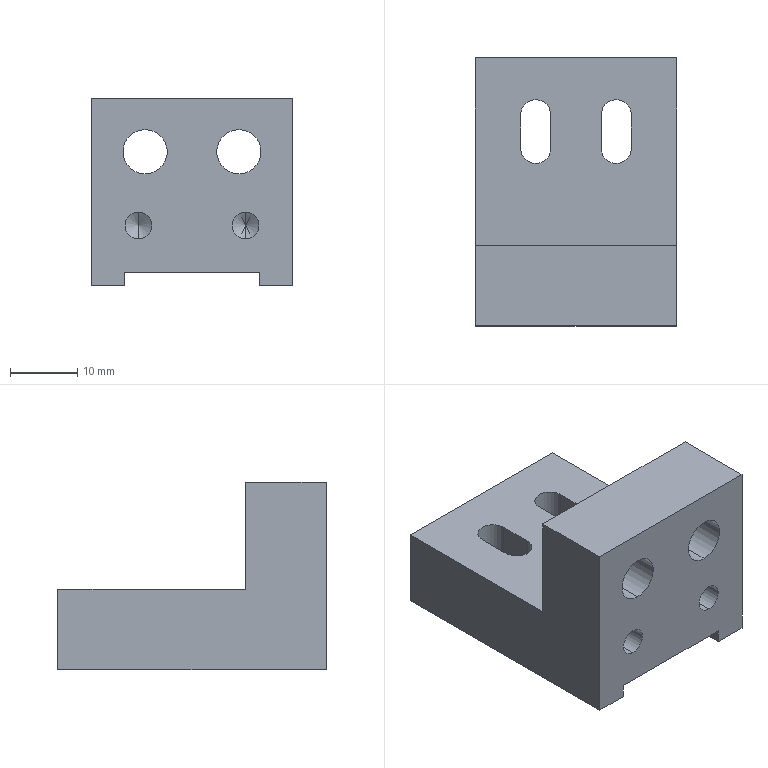Part | SolidWorks | features HoleWzd 4, ICE 3, Extrusion 1 | 1 solid | 38 faces | box 30 x 40 x 28 mm | volume 15981 mm3 | plane 18 | cylinder 16 | cone 4 | commonest cylinder face diameters 4 x4 4.5 x4 6.6 x4 11 x4
STEP:
#1=CARTESIAN_POINT('',(-7.,-14.4,14.5));
#2=VERTEX_POINT('',#1);
#3=CARTESIAN_POINT('',(-7.,-14.4,25.5));
#4=VERTEX_POINT('',#3);
#5=CARTESIAN_POINT('',(-7.,-14.4,20.));
#6=DIRECTION('',(0.,1.,0.));
#7=DIRECTION('',(0.,0.,1.));
#8=AXIS2_PLACEMENT_3D('',#5,#6,#7);
#9=CIRCLE('',#8,5.5);
#10=EDGE_CURVE('',#2,#4,#9,.T.);
#11=ORIENTED_EDGE('',*,*,#10,.F.);
#12=CARTESIAN_POINT('',(-7.,-8.,14.5));
#13=VERTEX_POINT('',#12);
#14=CARTESIAN_POINT('',(-7.,-8.,14.5));
#15=DIRECTION('',(0.,1.,0.));
#16=VECTOR('',#15,1000.);
#17=LINE('',#14,#16);
#18=EDGE_CURVE('',#2,#13,#17,.T.);
#19=ORIENTED_EDGE('',*,*,#18,.T.);
#20=CARTESIAN_POINT('',(-7.,-8.,25.5));
#21=VERTEX_POINT('',#20);
#22=CARTESIAN_POINT('',(-7.,-8.,20.));
#23=DIRECTION('',(0.,1.,0.));
#24=DIRECTION('',(0.,0.,1.));
#25=AXIS2_PLACEMENT_3D('',#22,#23,#24);
#26=CIRCLE('',#25,5.5);
#27=EDGE_CURVE('',#13,#21,#26,.T.);
#28=ORIENTED_EDGE('',*,*,#27,.T.);
#29=CARTESIAN_POINT('',(-7.,-8.,25.5));
#30=DIRECTION('',(0.,1.,0.));
#31=VECTOR('',#30,1000.);
#32=LINE('',#29,#31);
#33=EDGE_CURVE('',#4,#21,#32,.T.);
#34=ORIENTED_EDGE('',*,*,#33,.F.);
#35=EDGE_LOOP('',(#11,#19,#28,#34));
#36=FACE_OUTER_BOUND('',#35,.T.);
#37=CARTESIAN_POINT('',(-7.,-8.,20.));
#38=DIRECTION('',(0.,1.,0.));
#39=DIRECTION('',(0.,0.,1.));
#40=AXIS2_PLACEMENT_3D('',#37,#38,#39);
#41=CYLINDRICAL_SURFACE('',#40,5.5);
#42=ADVANCED_FACE('',(#36),#41,.F.);
#43=CARTESIAN_POINT('',(-7.,-20.,16.7));
#44=VERTEX_POINT('',#43);
#45=CARTESIAN_POINT('',(-7.,-20.,23.3));
#46=VERTEX_POINT('',#45);
#47=CARTESIAN_POINT('',(-7.,-20.,20.));
#48=DIRECTION('',(0.,1.,0.));
#49=DIRECTION('',(0.,0.,1.));
#50=AXIS2_PLACEMENT_3D('',#47,#48,#49);
#51=CIRCLE('',#50,3.3);
#52=EDGE_CURVE('',#44,#46,#51,.T.);
#53=ORIENTED_EDGE('',*,*,#52,.F.);
#54=CARTESIAN_POINT('',(-7.,-14.4,16.7));
#55=VERTEX_POINT('',#54);
#56=CARTESIAN_POINT('',(-7.,-8.,16.7));
#57=DIRECTION('',(0.,1.,0.));
#58=VECTOR('',#57,1000.);
#59=LINE('',#56,#58);
#60=EDGE_CURVE('',#44,#55,#59,.T.);
#61=ORIENTED_EDGE('',*,*,#60,.T.);
#62=CARTESIAN_POINT('',(-7.,-14.4,23.3));
#63=VERTEX_POINT('',#62);
#64=CARTESIAN_POINT('',(-7.,-14.4,20.));
#65=DIRECTION('',(0.,1.,0.));
#66=DIRECTION('',(0.,0.,1.));
#67=AXIS2_PLACEMENT_3D('',#64,#65,#66);
#68=CIRCLE('',#67,3.3);
#69=EDGE_CURVE('',#55,#63,#68,.T.);
#70=ORIENTED_EDGE('',*,*,#69,.T.);
#71=CARTESIAN_POINT('',(-7.,-8.,23.3));
#72=DIRECTION('',(0.,1.,0.));
#73=VECTOR('',#72,1000.);
#74=LINE('',#71,#73);
#75=EDGE_CURVE('',#46,#63,#74,.T.);
#76=ORIENTED_EDGE('',*,*,#75,.F.);
#77=EDGE_LOOP('',(#53,#61,#70,#76));
#78=FACE_OUTER_BOUND('',#77,.T.);
#79=CARTESIAN_POINT('',(-7.,-8.,20.));
#80=DIRECTION('',(0.,1.,0.));
#81=DIRECTION('',(0.,0.,1.));
#82=AXIS2_PLACEMENT_3D('',#79,#80,#81);
#83=CYLINDRICAL_SURFACE('',#82,3.3);
#84=ADVANCED_FACE('',(#78),#83,.F.);
#85=CARTESIAN_POINT('',(7.,-14.4,14.5));
#86=VERTEX_POINT('',#85);
#87=CARTESIAN_POINT('',(7.,-14.4,25.5));
#88=VERTEX_POINT('',#87);
#89=CARTESIAN_POINT('',(7.,-14.4,20.));
#90=DIRECTION('',(0.,1.,0.));
#91=DIRECTION('',(0.,0.,1.));
#92=AXIS2_PLACEMENT_3D('',#89,#90,#91);
#93=CIRCLE('',#92,5.5);
#94=EDGE_CURVE('',#86,#88,#93,.T.);
#95=ORIENTED_EDGE('',*,*,#94,.F.);
#96=CARTESIAN_POINT('',(7.,-8.,14.5));
#97=VERTEX_POINT('',#96);
#98=CARTESIAN_POINT('',(7.,-8.,14.5));
#99=DIRECTION('',(0.,1.,0.));
#100=VECTOR('',#99,1000.);
#101=LINE('',#98,#100);
#102=EDGE_CURVE('',#86,#97,#101,.T.);
#103=ORIENTED_EDGE('',*,*,#102,.T.);
#104=CARTESIAN_POINT('',(7.,-8.,25.5));
#105=VERTEX_POINT('',#104);
#106=CARTESIAN_POINT('',(7.,-8.,20.));
#107=DIRECTION('',(0.,1.,0.));
#108=DIRECTION('',(0.,0.,1.));
#109=AXIS2_PLACEMENT_3D('',#106,#107,#108);
#110=CIRCLE('',#109,5.5);
#111=EDGE_CURVE('',#97,#105,#110,.T.);
#112=ORIENTED_EDGE('',*,*,#111,.T.);
#113=CARTESIAN_POINT('',(7.,-8.,25.5));
#114=DIRECTION('',(0.,1.,0.));
#115=VECTOR('',#114,1000.);
#116=LINE('',#113,#115);
#117=EDGE_CURVE('',#88,#105,#116,.T.);
#118=ORIENTED_EDGE('',*,*,#117,.F.);
#119=EDGE_LOOP('',(#95,#103,#112,#118));
#120=FACE_OUTER_BOUND('',#119,.T.);
#121=CARTESIAN_POINT('',(7.,-8.,20.));
#122=DIRECTION('',(0.,1.,0.));
#123=DIRECTION('',(0.,0.,1.));
#124=AXIS2_PLACEMENT_3D('',#121,#122,#123);
#125=CYLINDRICAL_SURFACE('',#124,5.5);
#126=ADVANCED_FACE('',(#120),#125,.F.);
#127=CARTESIAN_POINT('',(7.,-20.,16.7));
#128=VERTEX_POINT('',#127);
#129=CARTESIAN_POINT('',(7.,-20.,23.3));
#130=VERTEX_POINT('',#129);
#131=CARTESIAN_POINT('',(7.,-20.,20.));
#132=DIRECTION('',(0.,1.,0.));
#133=DIRECTION('',(0.,0.,1.));
#134=AXIS2_PLACEMENT_3D('',#131,#132,#133);
#135=CIRCLE('',#134,3.3);
#136=EDGE_CURVE('',#128,#130,#135,.T.);
#137=ORIENTED_EDGE('',*,*,#136,.F.);
#138=CARTESIAN_POINT('',(7.,-14.4,16.7));
#139=VERTEX_POINT('',#138);
#140=CARTESIAN_POINT('',(7.,-8.,16.7));
#141=DIRECTION('',(0.,1.,0.));
#142=VECTOR('',#141,1000.);
#143=LINE('',#140,#142);
#144=EDGE_CURVE('',#128,#139,#143,.T.);
#145=ORIENTED_EDGE('',*,*,#144,.T.);
#146=CARTESIAN_POINT('',(7.,-14.4,23.3));
#147=VERTEX_POINT('',#146);
#148=CARTESIAN_POINT('',(7.,-14.4,20.));
#149=DIRECTION('',(0.,1.,0.));
#150=DIRECTION('',(0.,0.,1.));
#151=AXIS2_PLACEMENT_3D('',#148,#149,#150);
#152=CIRCLE('',#151,3.3);
#153=EDGE_CURVE('',#139,#147,#152,.T.);
#154=ORIENTED_EDGE('',*,*,#153,.T.);
#155=CARTESIAN_POINT('',(7.,-8.,23.3));
#156=DIRECTION('',(0.,1.,0.));
#157=VECTOR('',#156,1000.);
#158=LINE('',#155,#157);
#159=EDGE_CURVE('',#130,#147,#158,.T.);
#160=ORIENTED_EDGE('',*,*,#159,.F.);
#161=EDGE_LOOP('',(#137,#145,#154,#160));
#162=FACE_OUTER_BOUND('',#161,.T.);
#163=CARTESIAN_POINT('',(7.,-8.,20.));
#164=DIRECTION('',(0.,1.,0.));
#165=DIRECTION('',(0.,0.,1.));
#166=AXIS2_PLACEMENT_3D('',#163,#164,#165);
#167=CYLINDRICAL_SURFACE('',#166,3.3);
#168=ADVANCED_FACE('',(#162),#167,.F.);
#169=CARTESIAN_POINT('',(8.,-12.,11.));
#170=VERTEX_POINT('',#169);
#171=CARTESIAN_POINT('',(8.,-12.,7.));
#172=VERTEX_POINT('',#171);
#173=CARTESIAN_POINT('',(8.,-12.,9.));
#174=DIRECTION('',(0.,-1.,0.));
#175=DIRECTION('',(0.,0.,-1.));
#176=AXIS2_PLACEMENT_3D('',#173,#174,#175);
#177=CIRCLE('',#176,2.);
#178=EDGE_CURVE('',#170,#172,#177,.T.);
#179=ORIENTED_EDGE('',*,*,#178,.F.);
#180=CARTESIAN_POINT('',(8.,-20.,11.));
#181=VERTEX_POINT('',#180);
#182=CARTESIAN_POINT('',(8.,-20.,11.));
#183=DIRECTION('',(0.,-1.,0.));
#184=VECTOR('',#183,1000.);
#185=LINE('',#182,#184);
#186=EDGE_CURVE('',#170,#181,#185,.T.);
#187=ORIENTED_EDGE('',*,*,#186,.T.);
#188=CARTESIAN_POINT('',(8.,-20.,7.));
#189=VERTEX_POINT('',#188);
#190=CARTESIAN_POINT('',(8.,-20.,9.));
#191=DIRECTION('',(0.,-1.,0.));
#192=DIRECTION('',(0.,0.,-1.));
#193=AXIS2_PLACEMENT_3D('',#190,#191,#192);
#194=CIRCLE('',#193,2.);
#195=EDGE_CURVE('',#181,#189,#194,.T.);
#196=ORIENTED_EDGE('',*,*,#195,.T.);
#197=CARTESIAN_POINT('',(8.,-20.,7.));
#198=DIRECTION('',(0.,-1.,0.));
#199=VECTOR('',#198,1000.);
#200=LINE('',#197,#199);
#201=EDGE_CURVE('',#172,#189,#200,.T.);
#202=ORIENTED_EDGE('',*,*,#201,.F.);
#203=EDGE_LOOP('',(#179,#187,#196,#202));
#204=FACE_OUTER_BOUND('',#203,.T.);
#205=CARTESIAN_POINT('',(8.,-20.,9.));
#206=DIRECTION('',(0.,-1.,0.));
#207=DIRECTION('',(0.,0.,-1.));
#208=AXIS2_PLACEMENT_3D('',#205,#206,#207);
#209=CYLINDRICAL_SURFACE('',#208,2.);
#210=ADVANCED_FACE('',(#204),#209,.F.);
#211=CARTESIAN_POINT('',(8.,-10.798,9.));
#212=VERTEX_POINT('',#211);
#213=CARTESIAN_POINT('',(8.,-12.,7.));
#214=DIRECTION('',(0.,-0.515,-0.8572));
#215=VECTOR('',#214,1000.);
#216=LINE('',#213,#215);
#217=EDGE_CURVE('',#212,#172,#216,.T.);
#218=ORIENTED_EDGE('',*,*,#217,.F.);
#219=CARTESIAN_POINT('',(8.,-12.,11.));
#220=DIRECTION('',(0.,-0.515,0.8572));
#221=VECTOR('',#220,1000.);
#222=LINE('',#219,#221);
#223=EDGE_CURVE('',#212,#170,#222,.T.);
#224=ORIENTED_EDGE('',*,*,#223,.T.);
#225=ORIENTED_EDGE('',*,*,#178,.T.);
#226=EDGE_LOOP('',(#218,#224,#225));
#227=FACE_OUTER_BOUND('',#226,.T.);
#228=CARTESIAN_POINT('',(8.,-12.,9.));
#229=DIRECTION('',(0.,-1.,0.));
#230=DIRECTION('',(0.,0.,-1.));
#231=AXIS2_PLACEMENT_3D('',#228,#229,#230);
#232=CONICAL_SURFACE('',#231,2.,1.03);
#233=ADVANCED_FACE('',(#227),#232,.F.);
#234=CARTESIAN_POINT('',(-8.,-12.,11.));
#235=VERTEX_POINT('',#234);
#236=CARTESIAN_POINT('',(-8.,-12.,7.));
#237=VERTEX_POINT('',#236);
#238=CARTESIAN_POINT('',(-8.,-12.,9.));
#239=DIRECTION('',(0.,-1.,0.));
#240=DIRECTION('',(0.,0.,-1.));
#241=AXIS2_PLACEMENT_3D('',#238,#239,#240);
#242=CIRCLE('',#241,2.);
#243=EDGE_CURVE('',#235,#237,#242,.T.);
#244=ORIENTED_EDGE('',*,*,#243,.F.);
#245=CARTESIAN_POINT('',(-8.,-20.,11.));
#246=VERTEX_POINT('',#245);
#247=CARTESIAN_POINT('',(-8.,-20.,11.));
#248=DIRECTION('',(0.,-1.,0.));
#249=VECTOR('',#248,1000.);
#250=LINE('',#247,#249);
#251=EDGE_CURVE('',#235,#246,#250,.T.);
#252=ORIENTED_EDGE('',*,*,#251,.T.);
#253=CARTESIAN_POINT('',(-8.,-20.,7.));
#254=VERTEX_POINT('',#253);
#255=CARTESIAN_POINT('',(-8.,-20.,9.));
#256=DIRECTION('',(0.,-1.,0.));
#257=DIRECTION('',(0.,0.,-1.));
#258=AXIS2_PLACEMENT_3D('',#255,#256,#257);
#259=CIRCLE('',#258,2.);
#260=EDGE_CURVE('',#246,#254,#259,.T.);
#261=ORIENTED_EDGE('',*,*,#260,.T.);
#262=CARTESIAN_POINT('',(-8.,-20.,7.));
#263=DIRECTION('',(0.,-1.,0.));
#264=VECTOR('',#263,1000.);
#265=LINE('',#262,#264);
#266=EDGE_CURVE('',#237,#254,#265,.T.);
#267=ORIENTED_EDGE('',*,*,#266,.F.);
#268=EDGE_LOOP('',(#244,#252,#261,#267));
#269=FACE_OUTER_BOUND('',#268,.T.);
#270=CARTESIAN_POINT('',(-8.,-20.,9.));
#271=DIRECTION('',(0.,-1.,0.));
#272=DIRECTION('',(0.,0.,-1.));
#273=AXIS2_PLACEMENT_3D('',#270,#271,#272);
#274=CYLINDRICAL_SURFACE('',#273,2.);
#275=ADVANCED_FACE('',(#269),#274,.F.);
#276=CARTESIAN_POINT('',(-8.,-10.798,9.));
#277=VERTEX_POINT('',#276);
#278=CARTESIAN_POINT('',(-8.,-12.,7.));
#279=DIRECTION('',(0.,-0.515,-0.8572));
#280=VECTOR('',#279,1000.);
#281=LINE('',#278,#280);
#282=EDGE_CURVE('',#277,#237,#281,.T.);
#283=ORIENTED_EDGE('',*,*,#282,.F.);
#284=CARTESIAN_POINT('',(-8.,-12.,11.));
#285=DIRECTION('',(0.,-0.515,0.8572));
#286=VECTOR('',#285,1000.);
#287=LINE('',#284,#286);
#288=EDGE_CURVE('',#277,#235,#287,.T.);
#289=ORIENTED_EDGE('',*,*,#288,.T.);
#290=ORIENTED_EDGE('',*,*,#243,.T.);
#291=EDGE_LOOP('',(#283,#289,#290));
#292=FACE_OUTER_BOUND('',#291,.T.);
#293=CARTESIAN_POINT('',(-8.,-12.,9.));
#294=DIRECTION('',(0.,-1.,0.));
#295=DIRECTION('',(0.,0.,-1.));
#296=AXIS2_PLACEMENT_3D('',#293,#294,#295);
#297=CONICAL_SURFACE('',#296,2.,1.03);
#298=ADVANCED_FACE('',(#292),#297,.F.);
#299=CARTESIAN_POINT('',(-3.75,11.5,12.));
#300=VERTEX_POINT('',#299);
#301=CARTESIAN_POINT('',(-8.25,11.5,12.));
#302=VERTEX_POINT('',#301);
#303=CARTESIAN_POINT('',(-6.,11.5,12.));
#304=DIRECTION('',(0.,0.,1.));
#305=DIRECTION('',(1.,0.,0.));
#306=AXIS2_PLACEMENT_3D('',#303,#304,#305);
#307=CIRCLE('',#306,2.25);
#308=EDGE_CURVE('',#300,#302,#307,.T.);
#309=ORIENTED_EDGE('',*,*,#308,.F.);
#310=CARTESIAN_POINT('',(-3.75,6.5,12.));
#311=VERTEX_POINT('',#310);
#312=CARTESIAN_POINT('',(-3.75,6.5,12.));
#313=DIRECTION('',(0.,1.,0.));
#314=VECTOR('',#313,1000.);
#315=LINE('',#312,#314);
#316=EDGE_CURVE('',#311,#300,#315,.T.);
#317=ORIENTED_EDGE('',*,*,#316,.F.);
#318=CARTESIAN_POINT('',(-8.25,6.5,12.));
#319=VERTEX_POINT('',#318);
#320=CARTESIAN_POINT('',(-6.,6.5,12.));
#321=DIRECTION('',(0.,0.,1.));
#322=DIRECTION('',(1.,0.,0.));
#323=AXIS2_PLACEMENT_3D('',#320,#321,#322);
#324=CIRCLE('',#323,2.25);
#325=EDGE_CURVE('',#319,#311,#324,.T.);
#326=ORIENTED_EDGE('',*,*,#325,.F.);
#327=CARTESIAN_POINT('',(-8.25,6.5,12.));
#328=DIRECTION('',(0.,1.,0.));
#329=VECTOR('',#328,1000.);
#330=LINE('',#327,#329);
#331=EDGE_CURVE('',#319,#302,#330,.T.);
#332=ORIENTED_EDGE('',*,*,#331,.T.);
#333=EDGE_LOOP('',(#309,#317,#326,#332));
#334=FACE_BOUND('',#333,.T.);
#335=CARTESIAN_POINT('',(8.25,11.5,12.));
#336=VERTEX_POINT('',#335);
#337=CARTESIAN_POINT('',(3.75,11.5,12.));
#338=VERTEX_POINT('',#337);
#339=CARTESIAN_POINT('',(6.,11.5,12.));
#340=DIRECTION('',(0.,0.,1.));
#341=DIRECTION('',(1.,0.,0.));
#342=AXIS2_PLACEMENT_3D('',#339,#340,#341);
#343=CIRCLE('',#342,2.25);
#344=EDGE_CURVE('',#336,#338,#343,.T.);
#345=ORIENTED_EDGE('',*,*,#344,.F.);
#346=CARTESIAN_POINT('',(8.25,6.5,12.));
#347=VERTEX_POINT('',#346);
#348=CARTESIAN_POINT('',(8.25,6.5,12.));
#349=DIRECTION('',(0.,1.,0.));
#350=VECTOR('',#349,1000.);
#351=LINE('',#348,#350);
#352=EDGE_CURVE('',#347,#336,#351,.T.);
#353=ORIENTED_EDGE('',*,*,#352,.F.);
#354=CARTESIAN_POINT('',(3.75,6.5,12.));
#355=VERTEX_POINT('',#354);
#356=CARTESIAN_POINT('',(6.,6.5,12.));
#357=DIRECTION('',(0.,0.,1.));
#358=DIRECTION('',(1.,0.,0.));
#359=AXIS2_PLACEMENT_3D('',#356,#357,#358);
#360=CIRCLE('',#359,2.25);
#361=EDGE_CURVE('',#355,#347,#360,.T.);
#362=ORIENTED_EDGE('',*,*,#361,.F.);
#363=CARTESIAN_POINT('',(3.75,6.5,12.));
#364=DIRECTION('',(0.,1.,0.));
#365=VECTOR('',#364,1000.);
#366=LINE('',#363,#365);
#367=EDGE_CURVE('',#355,#338,#366,.T.);
#368=ORIENTED_EDGE('',*,*,#367,.T.);
#369=EDGE_LOOP('',(#345,#353,#362,#368));
#370=FACE_BOUND('',#369,.T.);
#371=CARTESIAN_POINT('',(-15.,20.,12.));
#372=VERTEX_POINT('',#371);
#373=CARTESIAN_POINT('',(-15.,-8.,12.));
#374=VERTEX_POINT('',#373);
#375=CARTESIAN_POINT('',(-15.,20.,12.));
#376=DIRECTION('',(0.,-1.,0.));
#377=VECTOR('',#376,1000.);
#378=LINE('',#375,#377);
#379=EDGE_CURVE('',#372,#374,#378,.T.);
#380=ORIENTED_EDGE('',*,*,#379,.T.);
#381=CARTESIAN_POINT('',(15.,-8.,12.));
#382=VERTEX_POINT('',#381);
#383=CARTESIAN_POINT('',(-15.,-8.,12.));
#384=DIRECTION('',(1.,0.,0.));
#385=VECTOR('',#384,1000.);
#386=LINE('',#383,#385);
#387=EDGE_CURVE('',#374,#382,#386,.T.);
#388=ORIENTED_EDGE('',*,*,#387,.T.);
#389=CARTESIAN_POINT('',(15.,20.,12.));
#390=VERTEX_POINT('',#389);
#391=CARTESIAN_POINT('',(15.,20.,12.));
#392=DIRECTION('',(0.,1.,0.));
#393=VECTOR('',#392,1000.);
#394=LINE('',#391,#393);
#395=EDGE_CURVE('',#382,#390,#394,.T.);
#396=ORIENTED_EDGE('',*,*,#395,.T.);
#397=CARTESIAN_POINT('',(-15.,20.,12.));
#398=DIRECTION('',(-1.,0.,0.));
#399=VECTOR('',#398,1000.);
#400=LINE('',#397,#399);
#401=EDGE_CURVE('',#390,#372,#400,.T.);
#402=ORIENTED_EDGE('',*,*,#401,.T.);
#403=EDGE_LOOP('',(#380,#388,#396,#402));
#404=FACE_OUTER_BOUND('',#403,.T.);
#405=CARTESIAN_POINT('',(0.,0.,12.));
#406=DIRECTION('',(0.,0.,1.));
#407=DIRECTION('',(1.,0.,0.));
#408=AXIS2_PLACEMENT_3D('',#405,#406,#407);
#409=PLANE('',#408);
#410=ADVANCED_FACE('',(#334,#370,#404),#409,.T.);
#411=CARTESIAN_POINT('',(-10.,20.,0.));
#412=VERTEX_POINT('',#411);
#413=CARTESIAN_POINT('',(-15.,20.,0.));
#414=VERTEX_POINT('',#413);
#415=CARTESIAN_POINT('',(-15.,20.,0.));
#416=DIRECTION('',(-1.,0.,0.));
#417=VECTOR('',#416,1000.);
#418=LINE('',#415,#417);
#419=EDGE_CURVE('',#412,#414,#418,.T.);
#420=ORIENTED_EDGE('',*,*,#419,.F.);
#421=CARTESIAN_POINT('',(-10.,-20.,0.));
#422=VERTEX_POINT('',#421);
#423=CARTESIAN_POINT('',(-10.,-20.,0.));
#424=DIRECTION('',(0.,1.,0.));
#425=VECTOR('',#424,1000.);
#426=LINE('',#423,#425);
#427=EDGE_CURVE('',#422,#412,#426,.T.);
#428=ORIENTED_EDGE('',*,*,#427,.F.);
#429=CARTESIAN_POINT('',(-15.,-20.,0.));
#430=VERTEX_POINT('',#429);
#431=CARTESIAN_POINT('',(-15.,-20.,0.));
#432=DIRECTION('',(1.,0.,0.));
#433=VECTOR('',#432,1000.);
#434=LINE('',#431,#433);
#435=EDGE_CURVE('',#430,#422,#434,.T.);
#436=ORIENTED_EDGE('',*,*,#435,.F.);
#437=CARTESIAN_POINT('',(-15.,20.,0.));
#438=DIRECTION('',(0.,-1.,0.));
#439=VECTOR('',#438,1000.);
#440=LINE('',#437,#439);
#441=EDGE_CURVE('',#414,#430,#440,.T.);
#442=ORIENTED_EDGE('',*,*,#441,.F.);
#443=EDGE_LOOP('',(#420,#428,#436,#442));
#444=FACE_OUTER_BOUND('',#443,.T.);
#445=CARTESIAN_POINT('',(0.,0.,0.));
#446=DIRECTION('',(0.,0.,1.));
#447=DIRECTION('',(1.,0.,0.));
#448=AXIS2_PLACEMENT_3D('',#445,#446,#447);
#449=PLANE('',#448);
#450=ADVANCED_FACE('',(#444),#449,.F.);
#451=CARTESIAN_POINT('',(15.,-20.,0.));
#452=VERTEX_POINT('',#451);
#453=CARTESIAN_POINT('',(15.,20.,0.));
#454=VERTEX_POINT('',#453);
#455=CARTESIAN_POINT('',(15.,20.,0.));
#456=DIRECTION('',(0.,1.,0.));
#457=VECTOR('',#456,1000.);
#458=LINE('',#455,#457);
#459=EDGE_CURVE('',#452,#454,#458,.T.);
#460=ORIENTED_EDGE('',*,*,#459,.T.);
#461=CARTESIAN_POINT('',(15.,20.,12.));
#462=DIRECTION('',(0.,0.,-1.));
#463=VECTOR('',#462,1000.);
#464=LINE('',#461,#463);
#465=EDGE_CURVE('',#390,#454,#464,.T.);
#466=ORIENTED_EDGE('',*,*,#465,.F.);
#467=ORIENTED_EDGE('',*,*,#395,.F.);
#468=CARTESIAN_POINT('',(15.,-8.,28.));
#469=VERTEX_POINT('',#468);
#470=CARTESIAN_POINT('',(15.,-8.,12.));
#471=DIRECTION('',(0.,0.,1.));
#472=VECTOR('',#471,1000.);
#473=LINE('',#470,#472);
#474=EDGE_CURVE('',#382,#469,#473,.T.);
#475=ORIENTED_EDGE('',*,*,#474,.T.);
#476=CARTESIAN_POINT('',(15.,-20.,28.));
#477=VERTEX_POINT('',#476);
#478=CARTESIAN_POINT('',(15.,-8.,28.));
#479=DIRECTION('',(0.,-1.,0.));
#480=VECTOR('',#479,1000.);
#481=LINE('',#478,#480);
#482=EDGE_CURVE('',#469,#477,#481,.T.);
#483=ORIENTED_EDGE('',*,*,#482,.T.);
#484=CARTESIAN_POINT('',(15.,-20.,12.));
#485=DIRECTION('',(0.,0.,-1.));
#486=VECTOR('',#485,1000.);
#487=LINE('',#484,#486);
#488=EDGE_CURVE('',#477,#452,#487,.T.);
#489=ORIENTED_EDGE('',*,*,#488,.T.);
#490=EDGE_LOOP('',(#460,#466,#467,#475,#483,#489));
#491=FACE_OUTER_BOUND('',#490,.T.);
#492=CARTESIAN_POINT('',(15.,20.,12.));
#493=DIRECTION('',(-1.,0.,0.));
#494=DIRECTION('',(0.,-1.,0.));
#495=AXIS2_PLACEMENT_3D('',#492,#493,#494);
#496=PLANE('',#495);
#497=ADVANCED_FACE('',(#491),#496,.F.);
#498=CARTESIAN_POINT('',(-10.,20.,2.));
#499=VERTEX_POINT('',#498);
#500=CARTESIAN_POINT('',(10.,20.,2.));
#501=VERTEX_POINT('',#500);
#502=CARTESIAN_POINT('',(-10.,20.,2.));
#503=DIRECTION('',(1.,0.,0.));
#504=VECTOR('',#503,1000.);
#505=LINE('',#502,#504);
#506=EDGE_CURVE('',#499,#501,#505,.T.);
#507=ORIENTED_EDGE('',*,*,#506,.F.);
#508=CARTESIAN_POINT('',(-10.,20.,0.));
#509=DIRECTION('',(0.,0.,1.));
#510=VECTOR('',#509,1000.);
#511=LINE('',#508,#510);
#512=EDGE_CURVE('',#412,#499,#511,.T.);
#513=ORIENTED_EDGE('',*,*,#512,.F.);
#514=ORIENTED_EDGE('',*,*,#419,.T.);
#515=CARTESIAN_POINT('',(-15.,20.,12.));
#516=DIRECTION('',(0.,0.,-1.));
#517=VECTOR('',#516,1000.);
#518=LINE('',#515,#517);
#519=EDGE_CURVE('',#372,#414,#518,.T.);
#520=ORIENTED_EDGE('',*,*,#519,.F.);
#521=ORIENTED_EDGE('',*,*,#401,.F.);
#522=ORIENTED_EDGE('',*,*,#465,.T.);
#523=CARTESIAN_POINT('',(10.,20.,0.));
#524=VERTEX_POINT('',#523);
#525=CARTESIAN_POINT('',(-15.,20.,0.));
#526=DIRECTION('',(-1.,0.,0.));
#527=VECTOR('',#526,1000.);
#528=LINE('',#525,#527);
#529=EDGE_CURVE('',#454,#524,#528,.T.);
#530=ORIENTED_EDGE('',*,*,#529,.T.);
#531=CARTESIAN_POINT('',(10.,20.,0.));
#532=DIRECTION('',(0.,0.,-1.));
#533=VECTOR('',#532,1000.);
#534=LINE('',#531,#533);
#535=EDGE_CURVE('',#501,#524,#534,.T.);
#536=ORIENTED_EDGE('',*,*,#535,.F.);
#537=EDGE_LOOP('',(#507,#513,#514,#520,#521,#522,#530,#536));
#538=FACE_OUTER_BOUND('',#537,.T.);
#539=CARTESIAN_POINT('',(-15.,20.,12.));
#540=DIRECTION('',(0.,-1.,0.));
#541=DIRECTION('',(0.,0.,-1.));
#542=AXIS2_PLACEMENT_3D('',#539,#540,#541);
#543=PLANE('',#542);
#544=ADVANCED_FACE('',(#538),#543,.F.);
#545=ORIENTED_EDGE('',*,*,#441,.T.);
#546=CARTESIAN_POINT('',(-15.,-20.,28.));
#547=VERTEX_POINT('',#546);
#548=CARTESIAN_POINT('',(-15.,-20.,12.));
#549=DIRECTION('',(0.,0.,-1.));
#550=VECTOR('',#549,1000.);
#551=LINE('',#548,#550);
#552=EDGE_CURVE('',#547,#430,#551,.T.);
#553=ORIENTED_EDGE('',*,*,#552,.F.);
#554=CARTESIAN_POINT('',(-15.,-8.,28.));
#555=VERTEX_POINT('',#554);
#556=CARTESIAN_POINT('',(-15.,-8.,28.));
#557=DIRECTION('',(0.,-1.,0.));
#558=VECTOR('',#557,1000.);
#559=LINE('',#556,#558);
#560=EDGE_CURVE('',#555,#547,#559,.T.);
#561=ORIENTED_EDGE('',*,*,#560,.F.);
#562=CARTESIAN_POINT('',(-15.,-8.,12.));
#563=DIRECTION('',(0.,0.,-1.));
#564=VECTOR('',#563,1000.);
#565=LINE('',#562,#564);
#566=EDGE_CURVE('',#555,#374,#565,.T.);
#567=ORIENTED_EDGE('',*,*,#566,.T.);
#568=ORIENTED_EDGE('',*,*,#379,.F.);
#569=ORIENTED_EDGE('',*,*,#519,.T.);
#570=EDGE_LOOP('',(#545,#553,#561,#567,#568,#569));
#571=FACE_OUTER_BOUND('',#570,.T.);
#572=CARTESIAN_POINT('',(-15.,20.,12.));
#573=DIRECTION('',(1.,0.,0.));
#574=DIRECTION('',(0.,1.,0.));
#575=AXIS2_PLACEMENT_3D('',#572,#573,#574);
#576=PLANE('',#575);
#577=ADVANCED_FACE('',(#571),#576,.F.);
#578=CARTESIAN_POINT('',(-7.,-20.,20.));
#579=DIRECTION('',(0.,1.,0.));
#580=DIRECTION('',(0.,0.,1.));
#581=AXIS2_PLACEMENT_3D('',#578,#579,#580);
#582=CIRCLE('',#581,3.3);
#583=EDGE_CURVE('',#46,#44,#582,.T.);
#584=ORIENTED_EDGE('',*,*,#583,.T.);
#585=ORIENTED_EDGE('',*,*,#52,.T.);
#586=EDGE_LOOP('',(#584,#585));
#587=FACE_BOUND('',#586,.T.);
#588=CARTESIAN_POINT('',(7.,-20.,20.));
#589=DIRECTION('',(0.,1.,0.));
#590=DIRECTION('',(0.,0.,1.));
#591=AXIS2_PLACEMENT_3D('',#588,#589,#590);
#592=CIRCLE('',#591,3.3);
#593=EDGE_CURVE('',#130,#128,#592,.T.);
#594=ORIENTED_EDGE('',*,*,#593,.T.);
#595=ORIENTED_EDGE('',*,*,#136,.T.);
#596=EDGE_LOOP('',(#594,#595));
#597=FACE_BOUND('',#596,.T.);
#598=CARTESIAN_POINT('',(8.,-20.,9.));
#599=DIRECTION('',(0.,-1.,0.));
#600=DIRECTION('',(0.,0.,-1.));
#601=AXIS2_PLACEMENT_3D('',#598,#599,#600);
#602=CIRCLE('',#601,2.);
#603=EDGE_CURVE('',#189,#181,#602,.T.);
#604=ORIENTED_EDGE('',*,*,#603,.F.);
#605=ORIENTED_EDGE('',*,*,#195,.F.);
#606=EDGE_LOOP('',(#604,#605));
#607=FACE_BOUND('',#606,.T.);
#608=CARTESIAN_POINT('',(-8.,-20.,9.));
#609=DIRECTION('',(0.,-1.,0.));
#610=DIRECTION('',(0.,0.,-1.));
#611=AXIS2_PLACEMENT_3D('',#608,#609,#610);
#612=CIRCLE('',#611,2.);
#613=EDGE_CURVE('',#254,#246,#612,.T.);
#614=ORIENTED_EDGE('',*,*,#613,.F.);
#615=ORIENTED_EDGE('',*,*,#260,.F.);
#616=EDGE_LOOP('',(#614,#615));
#617=FACE_BOUND('',#616,.T.);
#618=ORIENTED_EDGE('',*,*,#435,.T.);
#619=CARTESIAN_POINT('',(-10.,-20.,2.));
#620=VERTEX_POINT('',#619);
#621=CARTESIAN_POINT('',(-10.,-20.,0.));
#622=DIRECTION('',(0.,0.,1.));
#623=VECTOR('',#622,1000.);
#624=LINE('',#621,#623);
#625=EDGE_CURVE('',#422,#620,#624,.T.);
#626=ORIENTED_EDGE('',*,*,#625,.T.);
#627=CARTESIAN_POINT('',(10.,-20.,2.));
#628=VERTEX_POINT('',#627);
#629=CARTESIAN_POINT('',(-10.,-20.,2.));
#630=DIRECTION('',(1.,0.,0.));
#631=VECTOR('',#630,1000.);
#632=LINE('',#629,#631);
#633=EDGE_CURVE('',#620,#628,#632,.T.);
#634=ORIENTED_EDGE('',*,*,#633,.T.);
#635=CARTESIAN_POINT('',(10.,-20.,0.));
#636=VERTEX_POINT('',#635);
#637=CARTESIAN_POINT('',(10.,-20.,0.));
#638=DIRECTION('',(0.,0.,-1.));
#639=VECTOR('',#638,1000.);
#640=LINE('',#637,#639);
#641=EDGE_CURVE('',#628,#636,#640,.T.);
#642=ORIENTED_EDGE('',*,*,#641,.T.);
#643=CARTESIAN_POINT('',(-15.,-20.,0.));
#644=DIRECTION('',(1.,0.,0.));
#645=VECTOR('',#644,1000.);
#646=LINE('',#643,#645);
#647=EDGE_CURVE('',#636,#452,#646,.T.);
#648=ORIENTED_EDGE('',*,*,#647,.T.);
#649=ORIENTED_EDGE('',*,*,#488,.F.);
#650=CARTESIAN_POINT('',(-15.,-20.,28.));
#651=DIRECTION('',(-1.,0.,0.));
#652=VECTOR('',#651,1000.);
#653=LINE('',#650,#652);
#654=EDGE_CURVE('',#477,#547,#653,.T.);
#655=ORIENTED_EDGE('',*,*,#654,.T.);
#656=ORIENTED_EDGE('',*,*,#552,.T.);
#657=EDGE_LOOP('',(#618,#626,#634,#642,#648,#649,#655,#656));
#658=FACE_OUTER_BOUND('',#657,.T.);
#659=CARTESIAN_POINT('',(-15.,-20.,12.));
#660=DIRECTION('',(0.,1.,0.));
#661=DIRECTION('',(0.,0.,1.));
#662=AXIS2_PLACEMENT_3D('',#659,#660,#661);
#663=PLANE('',#662);
#664=ADVANCED_FACE('',(#587,#597,#607,#617,#658),#663,.F.);
#665=ORIENTED_EDGE('',*,*,#647,.F.);
#666=CARTESIAN_POINT('',(10.,-20.,0.));
#667=DIRECTION('',(0.,1.,0.));
#668=VECTOR('',#667,1000.);
#669=LINE('',#666,#668);
#670=EDGE_CURVE('',#636,#524,#669,.T.);
#671=ORIENTED_EDGE('',*,*,#670,.T.);
#672=ORIENTED_EDGE('',*,*,#529,.F.);
#673=ORIENTED_EDGE('',*,*,#459,.F.);
#674=EDGE_LOOP('',(#665,#671,#672,#673));
#675=FACE_OUTER_BOUND('',#674,.T.);
#676=CARTESIAN_POINT('',(0.,0.,0.));
#677=DIRECTION('',(0.,0.,1.));
#678=DIRECTION('',(1.,0.,0.));
#679=AXIS2_PLACEMENT_3D('',#676,#677,#678);
#680=PLANE('',#679);
#681=ADVANCED_FACE('',(#675),#680,.F.);
#682=ORIENTED_EDGE('',*,*,#512,.T.);
#683=CARTESIAN_POINT('',(-10.,-20.,2.));
#684=DIRECTION('',(0.,1.,0.));
#685=VECTOR('',#684,1000.);
#686=LINE('',#683,#685);
#687=EDGE_CURVE('',#620,#499,#686,.T.);
#688=ORIENTED_EDGE('',*,*,#687,.F.);
#689=ORIENTED_EDGE('',*,*,#625,.F.);
#690=ORIENTED_EDGE('',*,*,#427,.T.);
#691=EDGE_LOOP('',(#682,#688,#689,#690));
#692=FACE_OUTER_BOUND('',#691,.T.);
#693=CARTESIAN_POINT('',(-10.,-20.,0.));
#694=DIRECTION('',(-1.,0.,0.));
#695=DIRECTION('',(0.,0.,1.));
#696=AXIS2_PLACEMENT_3D('',#693,#694,#695);
#697=PLANE('',#696);
#698=ADVANCED_FACE('',(#692),#697,.F.);
#699=ORIENTED_EDGE('',*,*,#535,.T.);
#700=ORIENTED_EDGE('',*,*,#670,.F.);
#701=ORIENTED_EDGE('',*,*,#641,.F.);
#702=CARTESIAN_POINT('',(10.,-20.,2.));
#703=DIRECTION('',(0.,1.,0.));
#704=VECTOR('',#703,1000.);
#705=LINE('',#702,#704);
#706=EDGE_CURVE('',#628,#501,#705,.T.);
#707=ORIENTED_EDGE('',*,*,#706,.T.);
#708=EDGE_LOOP('',(#699,#700,#701,#707));
#709=FACE_OUTER_BOUND('',#708,.T.);
#710=CARTESIAN_POINT('',(10.,-20.,0.));
#711=DIRECTION('',(1.,0.,0.));
#712=DIRECTION('',(0.,0.,-1.));
#713=AXIS2_PLACEMENT_3D('',#710,#711,#712);
#714=PLANE('',#713);
#715=ADVANCED_FACE('',(#709),#714,.F.);
#716=CARTESIAN_POINT('',(-3.75,6.5,2.));
#717=VERTEX_POINT('',#716);
#718=CARTESIAN_POINT('',(-3.75,11.5,2.));
#719=VERTEX_POINT('',#718);
#720=CARTESIAN_POINT('',(-3.75,-20.,2.));
#721=DIRECTION('',(0.,1.,0.));
#722=VECTOR('',#721,1000.);
#723=LINE('',#720,#722);
#724=EDGE_CURVE('',#717,#719,#723,.T.);
#725=ORIENTED_EDGE('',*,*,#724,.T.);
#726=CARTESIAN_POINT('',(-8.25,11.5,2.));
#727=VERTEX_POINT('',#726);
#728=CARTESIAN_POINT('',(-6.,11.5,2.));
#729=DIRECTION('',(0.,0.,1.));
#730=DIRECTION('',(1.,0.,0.));
#731=AXIS2_PLACEMENT_3D('',#728,#729,#730);
#732=CIRCLE('',#731,2.25);
#733=EDGE_CURVE('',#719,#727,#732,.T.);
#734=ORIENTED_EDGE('',*,*,#733,.T.);
#735=CARTESIAN_POINT('',(-8.25,6.5,2.));
#736=VERTEX_POINT('',#735);
#737=CARTESIAN_POINT('',(-8.25,-20.,2.));
#738=DIRECTION('',(0.,-1.,0.));
#739=VECTOR('',#738,1000.);
#740=LINE('',#737,#739);
#741=EDGE_CURVE('',#727,#736,#740,.T.);
#742=ORIENTED_EDGE('',*,*,#741,.T.);
#743=CARTESIAN_POINT('',(-6.,6.5,2.));
#744=DIRECTION('',(0.,0.,1.));
#745=DIRECTION('',(1.,0.,0.));
#746=AXIS2_PLACEMENT_3D('',#743,#744,#745);
#747=CIRCLE('',#746,2.25);
#748=EDGE_CURVE('',#736,#717,#747,.T.);
#749=ORIENTED_EDGE('',*,*,#748,.T.);
#750=EDGE_LOOP('',(#725,#734,#742,#749));
#751=FACE_BOUND('',#750,.T.);
#752=CARTESIAN_POINT('',(8.25,11.5,2.));
#753=VERTEX_POINT('',#752);
#754=CARTESIAN_POINT('',(3.75,11.5,2.));
#755=VERTEX_POINT('',#754);
#756=CARTESIAN_POINT('',(6.,11.5,2.));
#757=DIRECTION('',(0.,0.,1.));
#758=DIRECTION('',(1.,0.,0.));
#759=AXIS2_PLACEMENT_3D('',#756,#757,#758);
#760=CIRCLE('',#759,2.25);
#761=EDGE_CURVE('',#753,#755,#760,.T.);
#762=ORIENTED_EDGE('',*,*,#761,.T.);
#763=CARTESIAN_POINT('',(3.75,6.5,2.));
#764=VERTEX_POINT('',#763);
#765=CARTESIAN_POINT('',(3.75,-20.,2.));
#766=DIRECTION('',(0.,-1.,0.));
#767=VECTOR('',#766,1000.);
#768=LINE('',#765,#767);
#769=EDGE_CURVE('',#755,#764,#768,.T.);
#770=ORIENTED_EDGE('',*,*,#769,.T.);
#771=CARTESIAN_POINT('',(8.25,6.5,2.));
#772=VERTEX_POINT('',#771);
#773=CARTESIAN_POINT('',(6.,6.5,2.));
#774=DIRECTION('',(0.,0.,1.));
#775=DIRECTION('',(1.,0.,0.));
#776=AXIS2_PLACEMENT_3D('',#773,#774,#775);
#777=CIRCLE('',#776,2.25);
#778=EDGE_CURVE('',#764,#772,#777,.T.);
#779=ORIENTED_EDGE('',*,*,#778,.T.);
#780=CARTESIAN_POINT('',(8.25,-20.,2.));
#781=DIRECTION('',(0.,1.,0.));
#782=VECTOR('',#781,1000.);
#783=LINE('',#780,#782);
#784=EDGE_CURVE('',#772,#753,#783,.T.);
#785=ORIENTED_EDGE('',*,*,#784,.T.);
#786=EDGE_LOOP('',(#762,#770,#779,#785));
#787=FACE_BOUND('',#786,.T.);
#788=ORIENTED_EDGE('',*,*,#506,.T.);
#789=ORIENTED_EDGE('',*,*,#706,.F.);
#790=ORIENTED_EDGE('',*,*,#633,.F.);
#791=ORIENTED_EDGE('',*,*,#687,.T.);
#792=EDGE_LOOP('',(#788,#789,#790,#791));
#793=FACE_OUTER_BOUND('',#792,.T.);
#794=CARTESIAN_POINT('',(-10.,-20.,2.));
#795=DIRECTION('',(0.,0.,1.));
#796=DIRECTION('',(1.,0.,0.));
#797=AXIS2_PLACEMENT_3D('',#794,#795,#796);
#798=PLANE('',#797);
#799=ADVANCED_FACE('',(#751,#787,#793),#798,.F.);
#800=CARTESIAN_POINT('',(3.75,11.5,12.));
#801=DIRECTION('',(0.,0.,1.));
#802=VECTOR('',#801,1000.);
#803=LINE('',#800,#802);
#804=EDGE_CURVE('',#755,#338,#803,.T.);
#805=ORIENTED_EDGE('',*,*,#804,.T.);
#806=ORIENTED_EDGE('',*,*,#367,.F.);
#807=CARTESIAN_POINT('',(3.75,6.5,12.));
#808=DIRECTION('',(0.,0.,-1.));
#809=VECTOR('',#808,1000.);
#810=LINE('',#807,#809);
#811=EDGE_CURVE('',#355,#764,#810,.T.);
#812=ORIENTED_EDGE('',*,*,#811,.T.);
#813=ORIENTED_EDGE('',*,*,#769,.F.);
#814=EDGE_LOOP('',(#805,#806,#812,#813));
#815=FACE_OUTER_BOUND('',#814,.T.);
#816=CARTESIAN_POINT('',(3.75,6.5,12.));
#817=DIRECTION('',(-1.,0.,0.));
#818=DIRECTION('',(0.,0.,1.));
#819=AXIS2_PLACEMENT_3D('',#816,#817,#818);
#820=PLANE('',#819);
#821=ADVANCED_FACE('',(#815),#820,.F.);
#822=CARTESIAN_POINT('',(8.25,11.5,0.));
#823=DIRECTION('',(0.,0.,-1.));
#824=VECTOR('',#823,1000.);
#825=LINE('',#822,#824);
#826=EDGE_CURVE('',#336,#753,#825,.T.);
#827=ORIENTED_EDGE('',*,*,#826,.F.);
#828=ORIENTED_EDGE('',*,*,#344,.T.);
#829=ORIENTED_EDGE('',*,*,#804,.F.);
#830=ORIENTED_EDGE('',*,*,#761,.F.);
#831=EDGE_LOOP('',(#827,#828,#829,#830));
#832=FACE_OUTER_BOUND('',#831,.T.);
#833=CARTESIAN_POINT('',(6.,11.5,12.));
#834=DIRECTION('',(0.,0.,1.));
#835=DIRECTION('',(1.,0.,0.));
#836=AXIS2_PLACEMENT_3D('',#833,#834,#835);
#837=CYLINDRICAL_SURFACE('',#836,2.25);
#838=ADVANCED_FACE('',(#832),#837,.F.);
#839=CARTESIAN_POINT('',(8.25,6.5,0.));
#840=DIRECTION('',(0.,0.,-1.));
#841=VECTOR('',#840,1000.);
#842=LINE('',#839,#841);
#843=EDGE_CURVE('',#347,#772,#842,.T.);
#844=ORIENTED_EDGE('',*,*,#843,.F.);
#845=ORIENTED_EDGE('',*,*,#352,.T.);
#846=ORIENTED_EDGE('',*,*,#826,.T.);
#847=ORIENTED_EDGE('',*,*,#784,.F.);
#848=EDGE_LOOP('',(#844,#845,#846,#847));
#849=FACE_OUTER_BOUND('',#848,.T.);
#850=CARTESIAN_POINT('',(8.25,6.5,0.));
#851=DIRECTION('',(1.,0.,0.));
#852=DIRECTION('',(0.,0.,-1.));
#853=AXIS2_PLACEMENT_3D('',#850,#851,#852);
#854=PLANE('',#853);
#855=ADVANCED_FACE('',(#849),#854,.F.);
#856=ORIENTED_EDGE('',*,*,#811,.F.);
#857=ORIENTED_EDGE('',*,*,#361,.T.);
#858=ORIENTED_EDGE('',*,*,#843,.T.);
#859=ORIENTED_EDGE('',*,*,#778,.F.);
#860=EDGE_LOOP('',(#856,#857,#858,#859));
#861=FACE_OUTER_BOUND('',#860,.T.);
#862=CARTESIAN_POINT('',(6.,6.5,12.));
#863=DIRECTION('',(0.,0.,1.));
#864=DIRECTION('',(1.,0.,0.));
#865=AXIS2_PLACEMENT_3D('',#862,#863,#864);
#866=CYLINDRICAL_SURFACE('',#865,2.25);
#867=ADVANCED_FACE('',(#861),#866,.F.);
#868=CARTESIAN_POINT('',(-3.75,11.5,0.));
#869=DIRECTION('',(0.,0.,-1.));
#870=VECTOR('',#869,1000.);
#871=LINE('',#868,#870);
#872=EDGE_CURVE('',#300,#719,#871,.T.);
#873=ORIENTED_EDGE('',*,*,#872,.F.);
#874=ORIENTED_EDGE('',*,*,#308,.T.);
#875=CARTESIAN_POINT('',(-8.25,11.5,12.));
#876=DIRECTION('',(0.,0.,1.));
#877=VECTOR('',#876,1000.);
#878=LINE('',#875,#877);
#879=EDGE_CURVE('',#727,#302,#878,.T.);
#880=ORIENTED_EDGE('',*,*,#879,.F.);
#881=ORIENTED_EDGE('',*,*,#733,.F.);
#882=EDGE_LOOP('',(#873,#874,#880,#881));
#883=FACE_OUTER_BOUND('',#882,.T.);
#884=CARTESIAN_POINT('',(-6.,11.5,12.));
#885=DIRECTION('',(0.,0.,1.));
#886=DIRECTION('',(1.,0.,0.));
#887=AXIS2_PLACEMENT_3D('',#884,#885,#886);
#888=CYLINDRICAL_SURFACE('',#887,2.25);
#889=ADVANCED_FACE('',(#883),#888,.F.);
#890=CARTESIAN_POINT('',(-3.75,6.5,0.));
#891=DIRECTION('',(0.,0.,-1.));
#892=VECTOR('',#891,1000.);
#893=LINE('',#890,#892);
#894=EDGE_CURVE('',#311,#717,#893,.T.);
#895=ORIENTED_EDGE('',*,*,#894,.F.);
#896=ORIENTED_EDGE('',*,*,#316,.T.);
#897=ORIENTED_EDGE('',*,*,#872,.T.);
#898=ORIENTED_EDGE('',*,*,#724,.F.);
#899=EDGE_LOOP('',(#895,#896,#897,#898));
#900=FACE_OUTER_BOUND('',#899,.T.);
#901=CARTESIAN_POINT('',(-3.75,6.5,0.));
#902=DIRECTION('',(1.,0.,0.));
#903=DIRECTION('',(0.,0.,-1.));
#904=AXIS2_PLACEMENT_3D('',#901,#902,#903);
#905=PLANE('',#904);
#906=ADVANCED_FACE('',(#900),#905,.F.);
#907=ORIENTED_EDGE('',*,*,#879,.T.);
#908=ORIENTED_EDGE('',*,*,#331,.F.);
#909=CARTESIAN_POINT('',(-8.25,6.5,12.));
#910=DIRECTION('',(0.,0.,-1.));
#911=VECTOR('',#910,1000.);
#912=LINE('',#909,#911);
#913=EDGE_CURVE('',#319,#736,#912,.T.);
#914=ORIENTED_EDGE('',*,*,#913,.T.);
#915=ORIENTED_EDGE('',*,*,#741,.F.);
#916=EDGE_LOOP('',(#907,#908,#914,#915));
#917=FACE_OUTER_BOUND('',#916,.T.);
#918=CARTESIAN_POINT('',(-8.25,6.5,12.));
#919=DIRECTION('',(-1.,0.,0.));
#920=DIRECTION('',(0.,0.,1.));
#921=AXIS2_PLACEMENT_3D('',#918,#919,#920);
#922=PLANE('',#921);
#923=ADVANCED_FACE('',(#917),#922,.F.);
#924=ORIENTED_EDGE('',*,*,#913,.F.);
#925=ORIENTED_EDGE('',*,*,#325,.T.);
#926=ORIENTED_EDGE('',*,*,#894,.T.);
#927=ORIENTED_EDGE('',*,*,#748,.F.);
#928=EDGE_LOOP('',(#924,#925,#926,#927));
#929=FACE_OUTER_BOUND('',#928,.T.);
#930=CARTESIAN_POINT('',(-6.,6.5,12.));
#931=DIRECTION('',(0.,0.,1.));
#932=DIRECTION('',(1.,0.,0.));
#933=AXIS2_PLACEMENT_3D('',#930,#931,#932);
#934=CYLINDRICAL_SURFACE('',#933,2.25);
#935=ADVANCED_FACE('',(#929),#934,.F.);
#936=ORIENTED_EDGE('',*,*,#654,.F.);
#937=ORIENTED_EDGE('',*,*,#482,.F.);
#938=CARTESIAN_POINT('',(-15.,-8.,28.));
#939=DIRECTION('',(-1.,0.,0.));
#940=VECTOR('',#939,1000.);
#941=LINE('',#938,#940);
#942=EDGE_CURVE('',#469,#555,#941,.T.);
#943=ORIENTED_EDGE('',*,*,#942,.T.);
#944=ORIENTED_EDGE('',*,*,#560,.T.);
#945=EDGE_LOOP('',(#936,#937,#943,#944));
#946=FACE_OUTER_BOUND('',#945,.T.);
#947=CARTESIAN_POINT('',(-15.,-8.,28.));
#948=DIRECTION('',(0.,0.,1.));
#949=DIRECTION('',(1.,0.,0.));
#950=AXIS2_PLACEMENT_3D('',#947,#948,#949);
#951=PLANE('',#950);
#952=ADVANCED_FACE('',(#946),#951,.T.);
#953=CARTESIAN_POINT('',(-7.,-8.,20.));
#954=DIRECTION('',(0.,1.,0.));
#955=DIRECTION('',(0.,0.,1.));
#956=AXIS2_PLACEMENT_3D('',#953,#954,#955);
#957=CIRCLE('',#956,5.5);
#958=EDGE_CURVE('',#21,#13,#957,.T.);
#959=ORIENTED_EDGE('',*,*,#958,.F.);
#960=ORIENTED_EDGE('',*,*,#27,.F.);
#961=EDGE_LOOP('',(#959,#960));
#962=FACE_BOUND('',#961,.T.);
#963=CARTESIAN_POINT('',(7.,-8.,20.));
#964=DIRECTION('',(0.,1.,0.));
#965=DIRECTION('',(0.,0.,1.));
#966=AXIS2_PLACEMENT_3D('',#963,#964,#965);
#967=CIRCLE('',#966,5.5);
#968=EDGE_CURVE('',#105,#97,#967,.T.);
#969=ORIENTED_EDGE('',*,*,#968,.F.);
#970=ORIENTED_EDGE('',*,*,#111,.F.);
#971=EDGE_LOOP('',(#969,#970));
#972=FACE_BOUND('',#971,.T.);
#973=ORIENTED_EDGE('',*,*,#566,.F.);
#974=ORIENTED_EDGE('',*,*,#942,.F.);
#975=ORIENTED_EDGE('',*,*,#474,.F.);
#976=ORIENTED_EDGE('',*,*,#387,.F.);
#977=EDGE_LOOP('',(#973,#974,#975,#976));
#978=FACE_OUTER_BOUND('',#977,.T.);
#979=CARTESIAN_POINT('',(0.,-8.,0.));
#980=DIRECTION('',(0.,1.,0.));
#981=DIRECTION('',(0.,0.,1.));
#982=AXIS2_PLACEMENT_3D('',#979,#980,#981);
#983=PLANE('',#982);
#984=ADVANCED_FACE('',(#962,#972,#978),#983,.T.);
#985=ORIENTED_EDGE('',*,*,#288,.F.);
#986=ORIENTED_EDGE('',*,*,#282,.T.);
#987=CARTESIAN_POINT('',(-8.,-12.,9.));
#988=DIRECTION('',(0.,-1.,0.));
#989=DIRECTION('',(0.,0.,-1.));
#990=AXIS2_PLACEMENT_3D('',#987,#988,#989);
#991=CIRCLE('',#990,2.);
#992=EDGE_CURVE('',#237,#235,#991,.T.);
#993=ORIENTED_EDGE('',*,*,#992,.T.);
#994=EDGE_LOOP('',(#985,#986,#993));
#995=FACE_OUTER_BOUND('',#994,.T.);
#996=CARTESIAN_POINT('',(-8.,-12.,9.));
#997=DIRECTION('',(0.,-1.,0.));
#998=DIRECTION('',(0.,0.,-1.));
#999=AXIS2_PLACEMENT_3D('',#996,#997,#998);
#1000=CONICAL_SURFACE('',#999,2.,1.03);
#1001=ADVANCED_FACE('',(#995),#1000,.F.);
#1002=ORIENTED_EDGE('',*,*,#251,.F.);
#1003=ORIENTED_EDGE('',*,*,#992,.F.);
#1004=ORIENTED_EDGE('',*,*,#266,.T.);
#1005=ORIENTED_EDGE('',*,*,#613,.T.);
#1006=EDGE_LOOP('',(#1002,#1003,#1004,#1005));
#1007=FACE_OUTER_BOUND('',#1006,.T.);
#1008=CARTESIAN_POINT('',(-8.,-20.,9.));
#1009=DIRECTION('',(0.,-1.,0.));
#1010=DIRECTION('',(0.,0.,-1.));
#1011=AXIS2_PLACEMENT_3D('',#1008,#1009,#1010);
#1012=CYLINDRICAL_SURFACE('',#1011,2.);
#1013=ADVANCED_FACE('',(#1007),#1012,.F.);
#1014=ORIENTED_EDGE('',*,*,#223,.F.);
#1015=ORIENTED_EDGE('',*,*,#217,.T.);
#1016=CARTESIAN_POINT('',(8.,-12.,9.));
#1017=DIRECTION('',(0.,-1.,0.));
#1018=DIRECTION('',(0.,0.,-1.));
#1019=AXIS2_PLACEMENT_3D('',#1016,#1017,#1018);
#1020=CIRCLE('',#1019,2.);
#1021=EDGE_CURVE('',#172,#170,#1020,.T.);
#1022=ORIENTED_EDGE('',*,*,#1021,.T.);
#1023=EDGE_LOOP('',(#1014,#1015,#1022));
#1024=FACE_OUTER_BOUND('',#1023,.T.);
#1025=CARTESIAN_POINT('',(8.,-12.,9.));
#1026=DIRECTION('',(0.,-1.,0.));
#1027=DIRECTION('',(0.,0.,-1.));
#1028=AXIS2_PLACEMENT_3D('',#1025,#1026,#1027);
#1029=CONICAL_SURFACE('',#1028,2.,1.03);
#1030=ADVANCED_FACE('',(#1024),#1029,.F.);
#1031=ORIENTED_EDGE('',*,*,#186,.F.);
#1032=ORIENTED_EDGE('',*,*,#1021,.F.);
#1033=ORIENTED_EDGE('',*,*,#201,.T.);
#1034=ORIENTED_EDGE('',*,*,#603,.T.);
#1035=EDGE_LOOP('',(#1031,#1032,#1033,#1034));
#1036=FACE_OUTER_BOUND('',#1035,.T.);
#1037=CARTESIAN_POINT('',(8.,-20.,9.));
#1038=DIRECTION('',(0.,-1.,0.));
#1039=DIRECTION('',(0.,0.,-1.));
#1040=AXIS2_PLACEMENT_3D('',#1037,#1038,#1039);
#1041=CYLINDRICAL_SURFACE('',#1040,2.);
#1042=ADVANCED_FACE('',(#1036),#1041,.F.);
#1043=ORIENTED_EDGE('',*,*,#144,.F.);
#1044=ORIENTED_EDGE('',*,*,#593,.F.);
#1045=ORIENTED_EDGE('',*,*,#159,.T.);
#1046=CARTESIAN_POINT('',(7.,-14.4,20.));
#1047=DIRECTION('',(0.,1.,0.));
#1048=DIRECTION('',(0.,0.,1.));
#1049=AXIS2_PLACEMENT_3D('',#1046,#1047,#1048);
#1050=CIRCLE('',#1049,3.3);
#1051=EDGE_CURVE('',#147,#139,#1050,.T.);
#1052=ORIENTED_EDGE('',*,*,#1051,.T.);
#1053=EDGE_LOOP('',(#1043,#1044,#1045,#1052));
#1054=FACE_OUTER_BOUND('',#1053,.T.);
#1055=CARTESIAN_POINT('',(7.,-8.,20.));
#1056=DIRECTION('',(0.,1.,0.));
#1057=DIRECTION('',(0.,0.,1.));
#1058=AXIS2_PLACEMENT_3D('',#1055,#1056,#1057);
#1059=CYLINDRICAL_SURFACE('',#1058,3.3);
#1060=ADVANCED_FACE('',(#1054),#1059,.F.);
#1061=ORIENTED_EDGE('',*,*,#1051,.F.);
#1062=ORIENTED_EDGE('',*,*,#153,.F.);
#1063=EDGE_LOOP('',(#1061,#1062));
#1064=FACE_BOUND('',#1063,.T.);
#1065=CARTESIAN_POINT('',(7.,-14.4,20.));
#1066=DIRECTION('',(0.,1.,0.));
#1067=DIRECTION('',(0.,0.,1.));
#1068=AXIS2_PLACEMENT_3D('',#1065,#1066,#1067);
#1069=CIRCLE('',#1068,5.5);
#1070=EDGE_CURVE('',#88,#86,#1069,.T.);
#1071=ORIENTED_EDGE('',*,*,#1070,.T.);
#1072=ORIENTED_EDGE('',*,*,#94,.T.);
#1073=EDGE_LOOP('',(#1071,#1072));
#1074=FACE_OUTER_BOUND('',#1073,.T.);
#1075=CARTESIAN_POINT('',(10.3,-14.4,20.));
#1076=DIRECTION('',(0.,-1.,0.));
#1077=DIRECTION('',(0.,0.,-1.));
#1078=AXIS2_PLACEMENT_3D('',#1075,#1076,#1077);
#1079=PLANE('',#1078);
#1080=ADVANCED_FACE('',(#1064,#1074),#1079,.F.);
#1081=ORIENTED_EDGE('',*,*,#102,.F.);
#1082=ORIENTED_EDGE('',*,*,#1070,.F.);
#1083=ORIENTED_EDGE('',*,*,#117,.T.);
#1084=ORIENTED_EDGE('',*,*,#968,.T.);
#1085=EDGE_LOOP('',(#1081,#1082,#1083,#1084));
#1086=FACE_OUTER_BOUND('',#1085,.T.);
#1087=CARTESIAN_POINT('',(7.,-8.,20.));
#1088=DIRECTION('',(0.,1.,0.));
#1089=DIRECTION('',(0.,0.,1.));
#1090=AXIS2_PLACEMENT_3D('',#1087,#1088,#1089);
#1091=CYLINDRICAL_SURFACE('',#1090,5.5);
#1092=ADVANCED_FACE('',(#1086),#1091,.F.);
#1093=ORIENTED_EDGE('',*,*,#60,.F.);
#1094=ORIENTED_EDGE('',*,*,#583,.F.);
#1095=ORIENTED_EDGE('',*,*,#75,.T.);
#1096=CARTESIAN_POINT('',(-7.,-14.4,20.));
#1097=DIRECTION('',(0.,1.,0.));
#1098=DIRECTION('',(0.,0.,1.));
#1099=AXIS2_PLACEMENT_3D('',#1096,#1097,#1098);
#1100=CIRCLE('',#1099,3.3);
#1101=EDGE_CURVE('',#63,#55,#1100,.T.);
#1102=ORIENTED_EDGE('',*,*,#1101,.T.);
#1103=EDGE_LOOP('',(#1093,#1094,#1095,#1102));
#1104=FACE_OUTER_BOUND('',#1103,.T.);
#1105=CARTESIAN_POINT('',(-7.,-8.,20.));
#1106=DIRECTION('',(0.,1.,0.));
#1107=DIRECTION('',(0.,0.,1.));
#1108=AXIS2_PLACEMENT_3D('',#1105,#1106,#1107);
#1109=CYLINDRICAL_SURFACE('',#1108,3.3);
#1110=ADVANCED_FACE('',(#1104),#1109,.F.);
#1111=ORIENTED_EDGE('',*,*,#1101,.F.);
#1112=ORIENTED_EDGE('',*,*,#69,.F.);
#1113=EDGE_LOOP('',(#1111,#1112));
#1114=FACE_BOUND('',#1113,.T.);
#1115=CARTESIAN_POINT('',(-7.,-14.4,20.));
#1116=DIRECTION('',(0.,1.,0.));
#1117=DIRECTION('',(0.,0.,1.));
#1118=AXIS2_PLACEMENT_3D('',#1115,#1116,#1117);
#1119=CIRCLE('',#1118,5.5);
#1120=EDGE_CURVE('',#4,#2,#1119,.T.);
#1121=ORIENTED_EDGE('',*,*,#1120,.T.);
#1122=ORIENTED_EDGE('',*,*,#10,.T.);
#1123=EDGE_LOOP('',(#1121,#1122));
#1124=FACE_OUTER_BOUND('',#1123,.T.);
#1125=CARTESIAN_POINT('',(-3.7,-14.4,20.));
#1126=DIRECTION('',(0.,-1.,0.));
#1127=DIRECTION('',(0.,0.,-1.));
#1128=AXIS2_PLACEMENT_3D('',#1125,#1126,#1127);
#1129=PLANE('',#1128);
#1130=ADVANCED_FACE('',(#1114,#1124),#1129,.F.);
#1131=ORIENTED_EDGE('',*,*,#18,.F.);
#1132=ORIENTED_EDGE('',*,*,#1120,.F.);
#1133=ORIENTED_EDGE('',*,*,#33,.T.);
#1134=ORIENTED_EDGE('',*,*,#958,.T.);
#1135=EDGE_LOOP('',(#1131,#1132,#1133,#1134));
#1136=FACE_OUTER_BOUND('',#1135,.T.);
#1137=CARTESIAN_POINT('',(-7.,-8.,20.));
#1138=DIRECTION('',(0.,1.,0.));
#1139=DIRECTION('',(0.,0.,1.));
#1140=AXIS2_PLACEMENT_3D('',#1137,#1138,#1139);
#1141=CYLINDRICAL_SURFACE('',#1140,5.5);
#1142=ADVANCED_FACE('',(#1136),#1141,.F.);
#1143=CLOSED_SHELL('',(#42,#84,#126,#168,#210,#233,#275,#298,#410,#450,#497,#544,#577,#664,#681,#698,#715,#799,#821,#838,#855,#867,#889,#906,#923,#935,#952,#984,#1001,#1013,#1030,#1042,#1060,#1080,#1092,#1110,#1130,#1142));
#1144=MANIFOLD_SOLID_BREP('',#1143);
#1145=CARTESIAN_POINT('',(0.,0.,0.));
#1146=DIRECTION('',(0.,0.,1.));
#1147=DIRECTION('',(1.,0.,0.));
#1148=AXIS2_PLACEMENT_3D('',#1145,#1146,#1147);
#1149=(LENGTH_UNIT()NAMED_UNIT(*)SI_UNIT(.MILLI.,.METRE.));
#1150=UNCERTAINTY_MEASURE_WITH_UNIT(LENGTH_MEASURE(0.00001),#1149,'','');
#1151=(NAMED_UNIT(*)PLANE_ANGLE_UNIT()SI_UNIT($,.RADIAN.));
#1152=(NAMED_UNIT(*)SI_UNIT($,.STERADIAN.)SOLID_ANGLE_UNIT());
#1153=(GEOMETRIC_REPRESENTATION_CONTEXT(3)GLOBAL_UNCERTAINTY_ASSIGNED_CONTEXT((#1150))GLOBAL_UNIT_ASSIGNED_CONTEXT((#1149,#1151,#1152))REPRESENTATION_CONTEXT('',''));
#1154=ADVANCED_BREP_SHAPE_REPRESENTATION('',(#1144,#1148),#1153);